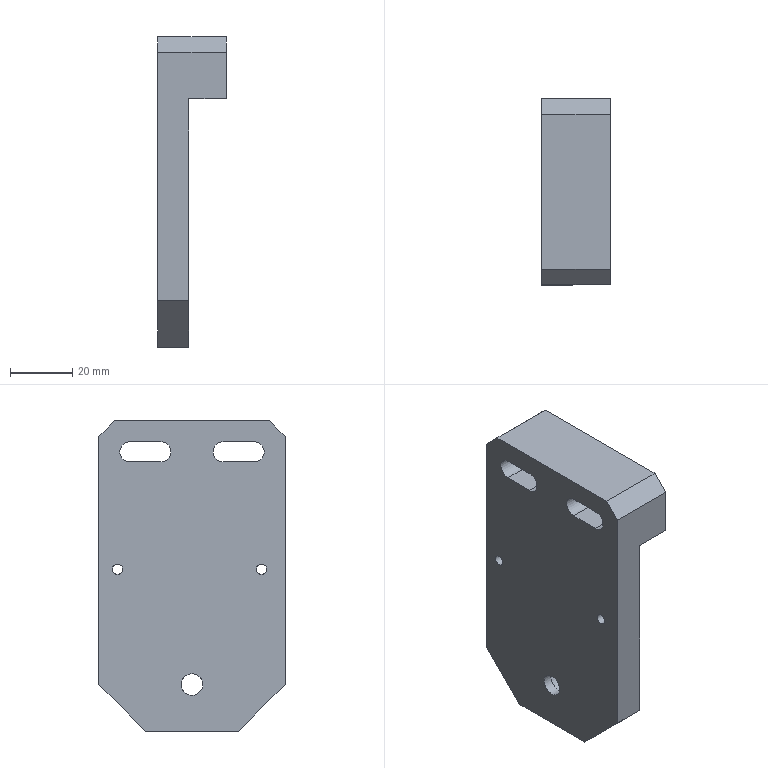Part | NX | features 5003_205_Bracket 2 | 1 solid | 25 faces | box 22 x 60 x 100 mm | volume 66444 mm3 | plane 17 | cylinder 8 | commonest cylinder face diameters 6.5 x4 3.3 x2 7 x1 10 x1
STEP:
#1=CARTESIAN_POINT('',(-243.475,-529.5,-147.));
#2=VERTEX_POINT('',#1);
#3=CARTESIAN_POINT('',(-243.475,-526.,-147.));
#4=DIRECTION('',(-1.,0.,0.));
#5=DIRECTION('',(0.,-1.,0.));
#6=AXIS2_PLACEMENT_3D('',#3,#4,#5);
#7=CIRCLE('',#6,3.5);
#8=EDGE_CURVE('',#2,#2,#7,.T.);
#9=ORIENTED_EDGE('',*,*,#8,.T.);
#10=EDGE_LOOP('',(#9));
#11=FACE_BOUND('',#10,.T.);
#12=CARTESIAN_POINT('',(-240.475,-526.,-143.5));
#13=VERTEX_POINT('',#12);
#14=CARTESIAN_POINT('',(-240.475,-526.,-147.));
#15=DIRECTION('',(1.,0.,0.));
#16=DIRECTION('',(0.,0.,1.));
#17=AXIS2_PLACEMENT_3D('',#14,#15,#16);
#18=CIRCLE('',#17,3.5);
#19=EDGE_CURVE('',#13,#13,#18,.T.);
#20=ORIENTED_EDGE('',*,*,#19,.T.);
#21=EDGE_LOOP('',(#20));
#22=FACE_BOUND('',#21,.T.);
#23=CARTESIAN_POINT('',(-243.475,-526.,-147.));
#24=DIRECTION('',(1.,0.,0.));
#25=DIRECTION('',(0.,1.,0.));
#26=AXIS2_PLACEMENT_3D('',#23,#24,#25);
#27=CYLINDRICAL_SURFACE('',#26,3.5);
#28=ADVANCED_FACE('',(#11,#22),#27,.F.);
#29=CARTESIAN_POINT('',(-243.475,-503.65,-109.85));
#30=VERTEX_POINT('',#29);
#31=CARTESIAN_POINT('',(-243.475,-502.,-109.85));
#32=DIRECTION('',(-1.,0.,0.));
#33=DIRECTION('',(0.,-1.,0.));
#34=AXIS2_PLACEMENT_3D('',#31,#32,#33);
#35=CIRCLE('',#34,1.65);
#36=EDGE_CURVE('',#30,#30,#35,.T.);
#37=ORIENTED_EDGE('',*,*,#36,.F.);
#38=EDGE_LOOP('',(#37));
#39=FACE_BOUND('',#38,.T.);
#40=CARTESIAN_POINT('',(-243.475,-550.05,-109.85));
#41=VERTEX_POINT('',#40);
#42=CARTESIAN_POINT('',(-243.475,-548.4,-109.85));
#43=DIRECTION('',(-1.,0.,0.));
#44=DIRECTION('',(0.,-1.,0.));
#45=AXIS2_PLACEMENT_3D('',#42,#43,#44);
#46=CIRCLE('',#45,1.65);
#47=EDGE_CURVE('',#41,#41,#46,.T.);
#48=ORIENTED_EDGE('',*,*,#47,.F.);
#49=EDGE_LOOP('',(#48));
#50=FACE_BOUND('',#49,.T.);
#51=CARTESIAN_POINT('',(-243.475,-551.,-62.));
#52=VERTEX_POINT('',#51);
#53=CARTESIAN_POINT('',(-243.475,-501.,-62.));
#54=VERTEX_POINT('',#53);
#55=CARTESIAN_POINT('',(-243.475,-496.,-62.));
#56=DIRECTION('',(0.,1.,0.));
#57=VECTOR('',#56,1000.);
#58=LINE('',#55,#57);
#59=EDGE_CURVE('',#52,#54,#58,.T.);
#60=ORIENTED_EDGE('',*,*,#59,.T.);
#61=CARTESIAN_POINT('',(-243.475,-496.,-67.));
#62=VERTEX_POINT('',#61);
#63=CARTESIAN_POINT('',(-243.475,-414.498,-148.502));
#64=DIRECTION('',(0.,-0.7071,0.7071));
#65=VECTOR('',#64,1000.);
#66=LINE('',#63,#65);
#67=EDGE_CURVE('',#54,#62,#66,.F.);
#68=ORIENTED_EDGE('',*,*,#67,.T.);
#69=CARTESIAN_POINT('',(-243.475,-496.,-147.));
#70=VERTEX_POINT('',#69);
#71=CARTESIAN_POINT('',(-243.475,-496.,-62.));
#72=DIRECTION('',(0.,0.,-1.));
#73=VECTOR('',#72,1000.);
#74=LINE('',#71,#73);
#75=EDGE_CURVE('',#62,#70,#74,.T.);
#76=ORIENTED_EDGE('',*,*,#75,.T.);
#77=CARTESIAN_POINT('',(-243.475,-511.,-162.));
#78=VERTEX_POINT('',#77);
#79=CARTESIAN_POINT('',(-243.475,-496.,-147.));
#80=DIRECTION('',(0.,-0.7071,-0.7071));
#81=VECTOR('',#80,1000.);
#82=LINE('',#79,#81);
#83=EDGE_CURVE('',#70,#78,#82,.T.);
#84=ORIENTED_EDGE('',*,*,#83,.T.);
#85=CARTESIAN_POINT('',(-243.475,-541.,-162.));
#86=VERTEX_POINT('',#85);
#87=CARTESIAN_POINT('',(-243.475,-511.,-162.));
#88=DIRECTION('',(0.,-1.,0.));
#89=VECTOR('',#88,1000.);
#90=LINE('',#87,#89);
#91=EDGE_CURVE('',#78,#86,#90,.T.);
#92=ORIENTED_EDGE('',*,*,#91,.T.);
#93=CARTESIAN_POINT('',(-243.475,-556.,-147.));
#94=VERTEX_POINT('',#93);
#95=CARTESIAN_POINT('',(-243.475,-541.,-162.));
#96=DIRECTION('',(0.,-0.7071,0.7071));
#97=VECTOR('',#96,1000.);
#98=LINE('',#95,#97);
#99=EDGE_CURVE('',#86,#94,#98,.T.);
#100=ORIENTED_EDGE('',*,*,#99,.T.);
#101=CARTESIAN_POINT('',(-243.475,-556.,-67.));
#102=VERTEX_POINT('',#101);
#103=CARTESIAN_POINT('',(-243.475,-556.,-62.));
#104=DIRECTION('',(0.,0.,1.));
#105=VECTOR('',#104,1000.);
#106=LINE('',#103,#105);
#107=EDGE_CURVE('',#94,#102,#106,.T.);
#108=ORIENTED_EDGE('',*,*,#107,.T.);
#109=CARTESIAN_POINT('',(-243.475,-615.498,-126.498));
#110=DIRECTION('',(0.,-0.7071,-0.7071));
#111=VECTOR('',#110,1000.);
#112=LINE('',#109,#111);
#113=EDGE_CURVE('',#102,#52,#112,.F.);
#114=ORIENTED_EDGE('',*,*,#113,.T.);
#115=EDGE_LOOP('',(#60,#68,#76,#84,#92,#100,#108,#114));
#116=FACE_BOUND('',#115,.T.);
#117=ORIENTED_EDGE('',*,*,#8,.F.);
#118=EDGE_LOOP('',(#117));
#119=FACE_BOUND('',#118,.T.);
#120=CARTESIAN_POINT('',(-243.475,-506.,-75.25));
#121=VERTEX_POINT('',#120);
#122=CARTESIAN_POINT('',(-243.475,-516.,-75.25));
#123=VERTEX_POINT('',#122);
#124=CARTESIAN_POINT('',(-243.475,-506.,-75.25));
#125=DIRECTION('',(0.,-1.,0.));
#126=VECTOR('',#125,1000.);
#127=LINE('',#124,#126);
#128=EDGE_CURVE('',#121,#123,#127,.T.);
#129=ORIENTED_EDGE('',*,*,#128,.F.);
#130=CARTESIAN_POINT('',(-243.475,-506.,-68.75));
#131=VERTEX_POINT('',#130);
#132=CARTESIAN_POINT('',(-243.475,-506.,-72.));
#133=DIRECTION('',(-1.,0.,0.));
#134=DIRECTION('',(0.,-1.,0.));
#135=AXIS2_PLACEMENT_3D('',#132,#133,#134);
#136=CIRCLE('',#135,3.25);
#137=EDGE_CURVE('',#131,#121,#136,.T.);
#138=ORIENTED_EDGE('',*,*,#137,.F.);
#139=CARTESIAN_POINT('',(-243.475,-516.,-68.75));
#140=VERTEX_POINT('',#139);
#141=CARTESIAN_POINT('',(-243.475,-506.,-68.75));
#142=DIRECTION('',(0.,1.,0.));
#143=VECTOR('',#142,1000.);
#144=LINE('',#141,#143);
#145=EDGE_CURVE('',#140,#131,#144,.T.);
#146=ORIENTED_EDGE('',*,*,#145,.F.);
#147=CARTESIAN_POINT('',(-243.475,-516.,-72.));
#148=DIRECTION('',(-1.,0.,0.));
#149=DIRECTION('',(0.,-1.,0.));
#150=AXIS2_PLACEMENT_3D('',#147,#148,#149);
#151=CIRCLE('',#150,3.25);
#152=EDGE_CURVE('',#123,#140,#151,.T.);
#153=ORIENTED_EDGE('',*,*,#152,.F.);
#154=EDGE_LOOP('',(#129,#138,#146,#153));
#155=FACE_BOUND('',#154,.T.);
#156=CARTESIAN_POINT('',(-243.475,-536.,-75.25));
#157=VERTEX_POINT('',#156);
#158=CARTESIAN_POINT('',(-243.475,-546.,-75.25));
#159=VERTEX_POINT('',#158);
#160=CARTESIAN_POINT('',(-243.475,-536.,-75.25));
#161=DIRECTION('',(0.,-1.,0.));
#162=VECTOR('',#161,1000.);
#163=LINE('',#160,#162);
#164=EDGE_CURVE('',#157,#159,#163,.T.);
#165=ORIENTED_EDGE('',*,*,#164,.F.);
#166=CARTESIAN_POINT('',(-243.475,-536.,-68.75));
#167=VERTEX_POINT('',#166);
#168=CARTESIAN_POINT('',(-243.475,-536.,-72.));
#169=DIRECTION('',(-1.,0.,0.));
#170=DIRECTION('',(0.,-1.,0.));
#171=AXIS2_PLACEMENT_3D('',#168,#169,#170);
#172=CIRCLE('',#171,3.25);
#173=EDGE_CURVE('',#167,#157,#172,.T.);
#174=ORIENTED_EDGE('',*,*,#173,.F.);
#175=CARTESIAN_POINT('',(-243.475,-546.,-68.75));
#176=VERTEX_POINT('',#175);
#177=CARTESIAN_POINT('',(-243.475,-536.,-68.75));
#178=DIRECTION('',(0.,1.,0.));
#179=VECTOR('',#178,1000.);
#180=LINE('',#177,#179);
#181=EDGE_CURVE('',#176,#167,#180,.T.);
#182=ORIENTED_EDGE('',*,*,#181,.F.);
#183=CARTESIAN_POINT('',(-243.475,-546.,-72.));
#184=DIRECTION('',(-1.,0.,0.));
#185=DIRECTION('',(0.,-1.,0.));
#186=AXIS2_PLACEMENT_3D('',#183,#184,#185);
#187=CIRCLE('',#186,3.25);
#188=EDGE_CURVE('',#159,#176,#187,.T.);
#189=ORIENTED_EDGE('',*,*,#188,.F.);
#190=EDGE_LOOP('',(#165,#174,#182,#189));
#191=FACE_BOUND('',#190,.T.);
#192=CARTESIAN_POINT('',(-243.475,-503.996,-238.));
#193=DIRECTION('',(-1.,0.,0.));
#194=DIRECTION('',(0.,-1.,0.));
#195=AXIS2_PLACEMENT_3D('',#192,#193,#194);
#196=PLANE('',#195);
#197=ADVANCED_FACE('',(#39,#50,#116,#119,#155,#191),#196,.T.);
#198=CARTESIAN_POINT('',(-221.475,-506.,-68.75));
#199=VERTEX_POINT('',#198);
#200=CARTESIAN_POINT('',(-221.475,-506.,-75.25));
#201=VERTEX_POINT('',#200);
#202=CARTESIAN_POINT('',(-221.475,-506.,-72.));
#203=DIRECTION('',(-1.,0.,0.));
#204=DIRECTION('',(0.,-1.,0.));
#205=AXIS2_PLACEMENT_3D('',#202,#203,#204);
#206=CIRCLE('',#205,3.25);
#207=EDGE_CURVE('',#199,#201,#206,.T.);
#208=ORIENTED_EDGE('',*,*,#207,.T.);
#209=CARTESIAN_POINT('',(-221.475,-516.,-75.25));
#210=VERTEX_POINT('',#209);
#211=CARTESIAN_POINT('',(-221.475,-506.,-75.25));
#212=DIRECTION('',(0.,-1.,0.));
#213=VECTOR('',#212,1000.);
#214=LINE('',#211,#213);
#215=EDGE_CURVE('',#201,#210,#214,.T.);
#216=ORIENTED_EDGE('',*,*,#215,.T.);
#217=CARTESIAN_POINT('',(-221.475,-516.,-68.75));
#218=VERTEX_POINT('',#217);
#219=CARTESIAN_POINT('',(-221.475,-516.,-72.));
#220=DIRECTION('',(-1.,0.,0.));
#221=DIRECTION('',(0.,-1.,0.));
#222=AXIS2_PLACEMENT_3D('',#219,#220,#221);
#223=CIRCLE('',#222,3.25);
#224=EDGE_CURVE('',#210,#218,#223,.T.);
#225=ORIENTED_EDGE('',*,*,#224,.T.);
#226=CARTESIAN_POINT('',(-221.475,-506.,-68.75));
#227=DIRECTION('',(0.,1.,0.));
#228=VECTOR('',#227,1000.);
#229=LINE('',#226,#228);
#230=EDGE_CURVE('',#218,#199,#229,.T.);
#231=ORIENTED_EDGE('',*,*,#230,.T.);
#232=EDGE_LOOP('',(#208,#216,#225,#231));
#233=FACE_BOUND('',#232,.T.);
#234=CARTESIAN_POINT('',(-221.475,-496.,-67.));
#235=VERTEX_POINT('',#234);
#236=CARTESIAN_POINT('',(-221.475,-496.,-82.));
#237=VERTEX_POINT('',#236);
#238=CARTESIAN_POINT('',(-221.475,-496.,-62.));
#239=DIRECTION('',(0.,0.,-1.));
#240=VECTOR('',#239,1000.);
#241=LINE('',#238,#240);
#242=EDGE_CURVE('',#235,#237,#241,.T.);
#243=ORIENTED_EDGE('',*,*,#242,.F.);
#244=CARTESIAN_POINT('',(-221.475,-501.,-62.));
#245=VERTEX_POINT('',#244);
#246=CARTESIAN_POINT('',(-221.475,-496.,-67.));
#247=DIRECTION('',(0.,0.7071,-0.7071));
#248=VECTOR('',#247,1000.);
#249=LINE('',#246,#248);
#250=EDGE_CURVE('',#235,#245,#249,.F.);
#251=ORIENTED_EDGE('',*,*,#250,.T.);
#252=CARTESIAN_POINT('',(-221.475,-551.,-62.));
#253=VERTEX_POINT('',#252);
#254=CARTESIAN_POINT('',(-221.475,-496.,-62.));
#255=DIRECTION('',(0.,1.,0.));
#256=VECTOR('',#255,1000.);
#257=LINE('',#254,#256);
#258=EDGE_CURVE('',#253,#245,#257,.T.);
#259=ORIENTED_EDGE('',*,*,#258,.F.);
#260=CARTESIAN_POINT('',(-221.475,-556.,-67.));
#261=VERTEX_POINT('',#260);
#262=CARTESIAN_POINT('',(-221.475,-551.,-62.));
#263=DIRECTION('',(0.,0.7071,0.7071));
#264=VECTOR('',#263,1000.);
#265=LINE('',#262,#264);
#266=EDGE_CURVE('',#253,#261,#265,.F.);
#267=ORIENTED_EDGE('',*,*,#266,.T.);
#268=CARTESIAN_POINT('',(-221.475,-556.,-82.));
#269=VERTEX_POINT('',#268);
#270=CARTESIAN_POINT('',(-221.475,-556.,-62.));
#271=DIRECTION('',(0.,0.,1.));
#272=VECTOR('',#271,1000.);
#273=LINE('',#270,#272);
#274=EDGE_CURVE('',#269,#261,#273,.T.);
#275=ORIENTED_EDGE('',*,*,#274,.F.);
#276=CARTESIAN_POINT('',(-221.475,-495.999,-82.));
#277=DIRECTION('',(0.,-1.,0.));
#278=VECTOR('',#277,1000.);
#279=LINE('',#276,#278);
#280=EDGE_CURVE('',#237,#269,#279,.T.);
#281=ORIENTED_EDGE('',*,*,#280,.F.);
#282=EDGE_LOOP('',(#243,#251,#259,#267,#275,#281));
#283=FACE_BOUND('',#282,.T.);
#284=CARTESIAN_POINT('',(-221.475,-536.,-68.75));
#285=VERTEX_POINT('',#284);
#286=CARTESIAN_POINT('',(-221.475,-536.,-75.25));
#287=VERTEX_POINT('',#286);
#288=CARTESIAN_POINT('',(-221.475,-536.,-72.));
#289=DIRECTION('',(-1.,0.,0.));
#290=DIRECTION('',(0.,-1.,0.));
#291=AXIS2_PLACEMENT_3D('',#288,#289,#290);
#292=CIRCLE('',#291,3.25);
#293=EDGE_CURVE('',#285,#287,#292,.T.);
#294=ORIENTED_EDGE('',*,*,#293,.T.);
#295=CARTESIAN_POINT('',(-221.475,-546.,-75.25));
#296=VERTEX_POINT('',#295);
#297=CARTESIAN_POINT('',(-221.475,-536.,-75.25));
#298=DIRECTION('',(0.,-1.,0.));
#299=VECTOR('',#298,1000.);
#300=LINE('',#297,#299);
#301=EDGE_CURVE('',#287,#296,#300,.T.);
#302=ORIENTED_EDGE('',*,*,#301,.T.);
#303=CARTESIAN_POINT('',(-221.475,-546.,-68.75));
#304=VERTEX_POINT('',#303);
#305=CARTESIAN_POINT('',(-221.475,-546.,-72.));
#306=DIRECTION('',(-1.,0.,0.));
#307=DIRECTION('',(0.,-1.,0.));
#308=AXIS2_PLACEMENT_3D('',#305,#306,#307);
#309=CIRCLE('',#308,3.25);
#310=EDGE_CURVE('',#296,#304,#309,.T.);
#311=ORIENTED_EDGE('',*,*,#310,.T.);
#312=CARTESIAN_POINT('',(-221.475,-536.,-68.75));
#313=DIRECTION('',(0.,1.,0.));
#314=VECTOR('',#313,1000.);
#315=LINE('',#312,#314);
#316=EDGE_CURVE('',#304,#285,#315,.T.);
#317=ORIENTED_EDGE('',*,*,#316,.T.);
#318=EDGE_LOOP('',(#294,#302,#311,#317));
#319=FACE_BOUND('',#318,.T.);
#320=CARTESIAN_POINT('',(-221.475,-503.996,-238.));
#321=DIRECTION('',(-1.,0.,0.));
#322=DIRECTION('',(0.,-1.,0.));
#323=AXIS2_PLACEMENT_3D('',#320,#321,#322);
#324=PLANE('',#323);
#325=ADVANCED_FACE('',(#233,#283,#319),#324,.F.);
#326=ORIENTED_EDGE('',*,*,#75,.F.);
#327=CARTESIAN_POINT('',(-243.475,-496.,-67.));
#328=DIRECTION('',(1.,0.,0.));
#329=VECTOR('',#328,1000.);
#330=LINE('',#327,#329);
#331=EDGE_CURVE('',#62,#235,#330,.T.);
#332=ORIENTED_EDGE('',*,*,#331,.T.);
#333=ORIENTED_EDGE('',*,*,#242,.T.);
#334=CARTESIAN_POINT('',(-233.475,-496.,-82.));
#335=VERTEX_POINT('',#334);
#336=CARTESIAN_POINT('',(-233.475,-496.,-82.));
#337=DIRECTION('',(1.,0.,0.));
#338=VECTOR('',#337,1000.);
#339=LINE('',#336,#338);
#340=EDGE_CURVE('',#335,#237,#339,.T.);
#341=ORIENTED_EDGE('',*,*,#340,.F.);
#342=CARTESIAN_POINT('',(-233.475,-496.,-147.));
#343=VERTEX_POINT('',#342);
#344=CARTESIAN_POINT('',(-233.475,-496.,-82.));
#345=DIRECTION('',(0.,0.,1.));
#346=VECTOR('',#345,1000.);
#347=LINE('',#344,#346);
#348=EDGE_CURVE('',#343,#335,#347,.T.);
#349=ORIENTED_EDGE('',*,*,#348,.F.);
#350=CARTESIAN_POINT('',(-243.475,-496.,-147.));
#351=DIRECTION('',(1.,0.,0.));
#352=VECTOR('',#351,1000.);
#353=LINE('',#350,#352);
#354=EDGE_CURVE('',#70,#343,#353,.T.);
#355=ORIENTED_EDGE('',*,*,#354,.F.);
#356=EDGE_LOOP('',(#326,#332,#333,#341,#349,#355));
#357=FACE_BOUND('',#356,.T.);
#358=CARTESIAN_POINT('',(-243.475,-496.,-62.));
#359=DIRECTION('',(0.,-1.,0.));
#360=DIRECTION('',(0.,0.,1.));
#361=AXIS2_PLACEMENT_3D('',#358,#359,#360);
#362=PLANE('',#361);
#363=ADVANCED_FACE('',(#357),#362,.F.);
#364=ORIENTED_EDGE('',*,*,#354,.T.);
#365=CARTESIAN_POINT('',(-233.475,-511.,-162.));
#366=VERTEX_POINT('',#365);
#367=CARTESIAN_POINT('',(-233.475,-463.499,-114.499));
#368=DIRECTION('',(0.,0.7071,0.7071));
#369=VECTOR('',#368,1000.);
#370=LINE('',#367,#369);
#371=EDGE_CURVE('',#366,#343,#370,.T.);
#372=ORIENTED_EDGE('',*,*,#371,.F.);
#373=CARTESIAN_POINT('',(-243.475,-511.,-162.));
#374=DIRECTION('',(1.,0.,0.));
#375=VECTOR('',#374,1000.);
#376=LINE('',#373,#375);
#377=EDGE_CURVE('',#78,#366,#376,.T.);
#378=ORIENTED_EDGE('',*,*,#377,.F.);
#379=ORIENTED_EDGE('',*,*,#83,.F.);
#380=EDGE_LOOP('',(#364,#372,#378,#379));
#381=FACE_BOUND('',#380,.T.);
#382=CARTESIAN_POINT('',(-243.475,-496.,-147.));
#383=DIRECTION('',(0.,-0.7071,0.7071));
#384=DIRECTION('',(0.,0.7071,0.7071));
#385=AXIS2_PLACEMENT_3D('',#382,#383,#384);
#386=PLANE('',#385);
#387=ADVANCED_FACE('',(#381),#386,.F.);
#388=ORIENTED_EDGE('',*,*,#377,.T.);
#389=CARTESIAN_POINT('',(-233.475,-541.,-162.));
#390=VERTEX_POINT('',#389);
#391=CARTESIAN_POINT('',(-233.475,-495.999,-162.));
#392=DIRECTION('',(0.,-1.,0.));
#393=VECTOR('',#392,1000.);
#394=LINE('',#391,#393);
#395=EDGE_CURVE('',#366,#390,#394,.T.);
#396=ORIENTED_EDGE('',*,*,#395,.T.);
#397=CARTESIAN_POINT('',(-243.475,-541.,-162.));
#398=DIRECTION('',(1.,0.,0.));
#399=VECTOR('',#398,1000.);
#400=LINE('',#397,#399);
#401=EDGE_CURVE('',#86,#390,#400,.T.);
#402=ORIENTED_EDGE('',*,*,#401,.F.);
#403=ORIENTED_EDGE('',*,*,#91,.F.);
#404=EDGE_LOOP('',(#388,#396,#402,#403));
#405=FACE_BOUND('',#404,.T.);
#406=CARTESIAN_POINT('',(-243.475,-511.,-162.));
#407=DIRECTION('',(0.,0.,1.));
#408=DIRECTION('',(-1.,0.,0.));
#409=AXIS2_PLACEMENT_3D('',#406,#407,#408);
#410=PLANE('',#409);
#411=ADVANCED_FACE('',(#405),#410,.F.);
#412=ORIENTED_EDGE('',*,*,#401,.T.);
#413=CARTESIAN_POINT('',(-233.475,-556.,-147.));
#414=VERTEX_POINT('',#413);
#415=CARTESIAN_POINT('',(-233.475,-558.499,-144.5));
#416=DIRECTION('',(0.,0.7071,-0.7071));
#417=VECTOR('',#416,1000.);
#418=LINE('',#415,#417);
#419=EDGE_CURVE('',#414,#390,#418,.T.);
#420=ORIENTED_EDGE('',*,*,#419,.F.);
#421=CARTESIAN_POINT('',(-243.475,-556.,-147.));
#422=DIRECTION('',(1.,0.,0.));
#423=VECTOR('',#422,1000.);
#424=LINE('',#421,#423);
#425=EDGE_CURVE('',#94,#414,#424,.T.);
#426=ORIENTED_EDGE('',*,*,#425,.F.);
#427=ORIENTED_EDGE('',*,*,#99,.F.);
#428=EDGE_LOOP('',(#412,#420,#426,#427));
#429=FACE_BOUND('',#428,.T.);
#430=CARTESIAN_POINT('',(-243.475,-541.,-162.));
#431=DIRECTION('',(0.,0.7071,0.7071));
#432=DIRECTION('',(0.,0.7071,-0.7071));
#433=AXIS2_PLACEMENT_3D('',#430,#431,#432);
#434=PLANE('',#433);
#435=ADVANCED_FACE('',(#429),#434,.F.);
#436=ORIENTED_EDGE('',*,*,#274,.T.);
#437=CARTESIAN_POINT('',(-243.475,-556.,-67.));
#438=DIRECTION('',(-1.,0.,0.));
#439=VECTOR('',#438,1000.);
#440=LINE('',#437,#439);
#441=EDGE_CURVE('',#261,#102,#440,.T.);
#442=ORIENTED_EDGE('',*,*,#441,.T.);
#443=ORIENTED_EDGE('',*,*,#107,.F.);
#444=ORIENTED_EDGE('',*,*,#425,.T.);
#445=CARTESIAN_POINT('',(-233.475,-556.,-82.));
#446=VERTEX_POINT('',#445);
#447=CARTESIAN_POINT('',(-233.475,-556.,-82.));
#448=DIRECTION('',(0.,0.,-1.));
#449=VECTOR('',#448,1000.);
#450=LINE('',#447,#449);
#451=EDGE_CURVE('',#446,#414,#450,.T.);
#452=ORIENTED_EDGE('',*,*,#451,.F.);
#453=CARTESIAN_POINT('',(-233.475,-556.,-82.));
#454=DIRECTION('',(-1.,0.,0.));
#455=VECTOR('',#454,1000.);
#456=LINE('',#453,#455);
#457=EDGE_CURVE('',#269,#446,#456,.T.);
#458=ORIENTED_EDGE('',*,*,#457,.F.);
#459=EDGE_LOOP('',(#436,#442,#443,#444,#452,#458));
#460=FACE_BOUND('',#459,.T.);
#461=CARTESIAN_POINT('',(-243.475,-556.,-62.));
#462=DIRECTION('',(0.,1.,0.));
#463=DIRECTION('',(0.,0.,-1.));
#464=AXIS2_PLACEMENT_3D('',#461,#462,#463);
#465=PLANE('',#464);
#466=ADVANCED_FACE('',(#460),#465,.F.);
#467=ORIENTED_EDGE('',*,*,#258,.T.);
#468=CARTESIAN_POINT('',(-243.475,-501.,-62.));
#469=DIRECTION('',(-1.,0.,0.));
#470=VECTOR('',#469,1000.);
#471=LINE('',#468,#470);
#472=EDGE_CURVE('',#245,#54,#471,.T.);
#473=ORIENTED_EDGE('',*,*,#472,.T.);
#474=ORIENTED_EDGE('',*,*,#59,.F.);
#475=CARTESIAN_POINT('',(-243.475,-551.,-62.));
#476=DIRECTION('',(1.,0.,0.));
#477=VECTOR('',#476,1000.);
#478=LINE('',#475,#477);
#479=EDGE_CURVE('',#52,#253,#478,.T.);
#480=ORIENTED_EDGE('',*,*,#479,.T.);
#481=EDGE_LOOP('',(#467,#473,#474,#480));
#482=FACE_BOUND('',#481,.T.);
#483=CARTESIAN_POINT('',(-243.475,-496.,-62.));
#484=DIRECTION('',(0.,0.,-1.));
#485=DIRECTION('',(1.,0.,0.));
#486=AXIS2_PLACEMENT_3D('',#483,#484,#485);
#487=PLANE('',#486);
#488=ADVANCED_FACE('',(#482),#487,.F.);
#489=ORIENTED_EDGE('',*,*,#207,.F.);
#490=CARTESIAN_POINT('',(-243.475,-506.,-68.75));
#491=DIRECTION('',(1.,0.,0.));
#492=VECTOR('',#491,1000.);
#493=LINE('',#490,#492);
#494=EDGE_CURVE('',#131,#199,#493,.T.);
#495=ORIENTED_EDGE('',*,*,#494,.F.);
#496=ORIENTED_EDGE('',*,*,#137,.T.);
#497=CARTESIAN_POINT('',(-243.475,-506.,-75.25));
#498=DIRECTION('',(1.,0.,0.));
#499=VECTOR('',#498,1000.);
#500=LINE('',#497,#499);
#501=EDGE_CURVE('',#121,#201,#500,.T.);
#502=ORIENTED_EDGE('',*,*,#501,.T.);
#503=EDGE_LOOP('',(#489,#495,#496,#502));
#504=FACE_BOUND('',#503,.T.);
#505=CARTESIAN_POINT('',(-243.475,-506.,-72.));
#506=DIRECTION('',(1.,0.,0.));
#507=DIRECTION('',(0.,1.,0.));
#508=AXIS2_PLACEMENT_3D('',#505,#506,#507);
#509=CYLINDRICAL_SURFACE('',#508,3.25);
#510=ADVANCED_FACE('',(#504),#509,.F.);
#511=ORIENTED_EDGE('',*,*,#215,.F.);
#512=ORIENTED_EDGE('',*,*,#501,.F.);
#513=ORIENTED_EDGE('',*,*,#128,.T.);
#514=CARTESIAN_POINT('',(-243.475,-516.,-75.25));
#515=DIRECTION('',(1.,0.,0.));
#516=VECTOR('',#515,1000.);
#517=LINE('',#514,#516);
#518=EDGE_CURVE('',#123,#210,#517,.T.);
#519=ORIENTED_EDGE('',*,*,#518,.T.);
#520=EDGE_LOOP('',(#511,#512,#513,#519));
#521=FACE_BOUND('',#520,.T.);
#522=CARTESIAN_POINT('',(-243.475,-506.,-75.25));
#523=DIRECTION('',(0.,0.,1.));
#524=DIRECTION('',(-1.,0.,0.));
#525=AXIS2_PLACEMENT_3D('',#522,#523,#524);
#526=PLANE('',#525);
#527=ADVANCED_FACE('',(#521),#526,.T.);
#528=ORIENTED_EDGE('',*,*,#224,.F.);
#529=ORIENTED_EDGE('',*,*,#518,.F.);
#530=ORIENTED_EDGE('',*,*,#152,.T.);
#531=CARTESIAN_POINT('',(-243.475,-516.,-68.75));
#532=DIRECTION('',(1.,0.,0.));
#533=VECTOR('',#532,1000.);
#534=LINE('',#531,#533);
#535=EDGE_CURVE('',#140,#218,#534,.T.);
#536=ORIENTED_EDGE('',*,*,#535,.T.);
#537=EDGE_LOOP('',(#528,#529,#530,#536));
#538=FACE_BOUND('',#537,.T.);
#539=CARTESIAN_POINT('',(-243.475,-516.,-72.));
#540=DIRECTION('',(1.,0.,0.));
#541=DIRECTION('',(0.,1.,0.));
#542=AXIS2_PLACEMENT_3D('',#539,#540,#541);
#543=CYLINDRICAL_SURFACE('',#542,3.25);
#544=ADVANCED_FACE('',(#538),#543,.F.);
#545=ORIENTED_EDGE('',*,*,#230,.F.);
#546=ORIENTED_EDGE('',*,*,#535,.F.);
#547=ORIENTED_EDGE('',*,*,#145,.T.);
#548=ORIENTED_EDGE('',*,*,#494,.T.);
#549=EDGE_LOOP('',(#545,#546,#547,#548));
#550=FACE_BOUND('',#549,.T.);
#551=CARTESIAN_POINT('',(-243.475,-506.,-68.75));
#552=DIRECTION('',(0.,0.,-1.));
#553=DIRECTION('',(1.,0.,0.));
#554=AXIS2_PLACEMENT_3D('',#551,#552,#553);
#555=PLANE('',#554);
#556=ADVANCED_FACE('',(#550),#555,.T.);
#557=ORIENTED_EDGE('',*,*,#293,.F.);
#558=CARTESIAN_POINT('',(-243.475,-536.,-68.75));
#559=DIRECTION('',(1.,0.,0.));
#560=VECTOR('',#559,1000.);
#561=LINE('',#558,#560);
#562=EDGE_CURVE('',#167,#285,#561,.T.);
#563=ORIENTED_EDGE('',*,*,#562,.F.);
#564=ORIENTED_EDGE('',*,*,#173,.T.);
#565=CARTESIAN_POINT('',(-243.475,-536.,-75.25));
#566=DIRECTION('',(1.,0.,0.));
#567=VECTOR('',#566,1000.);
#568=LINE('',#565,#567);
#569=EDGE_CURVE('',#157,#287,#568,.T.);
#570=ORIENTED_EDGE('',*,*,#569,.T.);
#571=EDGE_LOOP('',(#557,#563,#564,#570));
#572=FACE_BOUND('',#571,.T.);
#573=CARTESIAN_POINT('',(-243.475,-536.,-72.));
#574=DIRECTION('',(1.,0.,0.));
#575=DIRECTION('',(0.,1.,0.));
#576=AXIS2_PLACEMENT_3D('',#573,#574,#575);
#577=CYLINDRICAL_SURFACE('',#576,3.25);
#578=ADVANCED_FACE('',(#572),#577,.F.);
#579=ORIENTED_EDGE('',*,*,#301,.F.);
#580=ORIENTED_EDGE('',*,*,#569,.F.);
#581=ORIENTED_EDGE('',*,*,#164,.T.);
#582=CARTESIAN_POINT('',(-243.475,-546.,-75.25));
#583=DIRECTION('',(1.,0.,0.));
#584=VECTOR('',#583,1000.);
#585=LINE('',#582,#584);
#586=EDGE_CURVE('',#159,#296,#585,.T.);
#587=ORIENTED_EDGE('',*,*,#586,.T.);
#588=EDGE_LOOP('',(#579,#580,#581,#587));
#589=FACE_BOUND('',#588,.T.);
#590=CARTESIAN_POINT('',(-243.475,-536.,-75.25));
#591=DIRECTION('',(0.,0.,1.));
#592=DIRECTION('',(-1.,0.,0.));
#593=AXIS2_PLACEMENT_3D('',#590,#591,#592);
#594=PLANE('',#593);
#595=ADVANCED_FACE('',(#589),#594,.T.);
#596=ORIENTED_EDGE('',*,*,#310,.F.);
#597=ORIENTED_EDGE('',*,*,#586,.F.);
#598=ORIENTED_EDGE('',*,*,#188,.T.);
#599=CARTESIAN_POINT('',(-243.475,-546.,-68.75));
#600=DIRECTION('',(1.,0.,0.));
#601=VECTOR('',#600,1000.);
#602=LINE('',#599,#601);
#603=EDGE_CURVE('',#176,#304,#602,.T.);
#604=ORIENTED_EDGE('',*,*,#603,.T.);
#605=EDGE_LOOP('',(#596,#597,#598,#604));
#606=FACE_BOUND('',#605,.T.);
#607=CARTESIAN_POINT('',(-243.475,-546.,-72.));
#608=DIRECTION('',(1.,0.,0.));
#609=DIRECTION('',(0.,1.,0.));
#610=AXIS2_PLACEMENT_3D('',#607,#608,#609);
#611=CYLINDRICAL_SURFACE('',#610,3.25);
#612=ADVANCED_FACE('',(#606),#611,.F.);
#613=ORIENTED_EDGE('',*,*,#316,.F.);
#614=ORIENTED_EDGE('',*,*,#603,.F.);
#615=ORIENTED_EDGE('',*,*,#181,.T.);
#616=ORIENTED_EDGE('',*,*,#562,.T.);
#617=EDGE_LOOP('',(#613,#614,#615,#616));
#618=FACE_BOUND('',#617,.T.);
#619=CARTESIAN_POINT('',(-243.475,-536.,-68.75));
#620=DIRECTION('',(0.,0.,-1.));
#621=DIRECTION('',(1.,0.,0.));
#622=AXIS2_PLACEMENT_3D('',#619,#620,#621);
#623=PLANE('',#622);
#624=ADVANCED_FACE('',(#618),#623,.T.);
#625=CARTESIAN_POINT('',(-233.475,-502.,-111.5));
#626=VERTEX_POINT('',#625);
#627=CARTESIAN_POINT('',(-233.475,-502.,-109.85));
#628=DIRECTION('',(-1.,0.,0.));
#629=DIRECTION('',(0.,0.,-1.));
#630=AXIS2_PLACEMENT_3D('',#627,#628,#629);
#631=CIRCLE('',#630,1.65);
#632=EDGE_CURVE('',#626,#626,#631,.T.);
#633=ORIENTED_EDGE('',*,*,#632,.T.);
#634=EDGE_LOOP('',(#633));
#635=FACE_BOUND('',#634,.T.);
#636=CARTESIAN_POINT('',(-233.475,-548.4,-111.5));
#637=VERTEX_POINT('',#636);
#638=CARTESIAN_POINT('',(-233.475,-548.4,-109.85));
#639=DIRECTION('',(-1.,0.,0.));
#640=DIRECTION('',(0.,0.,-1.));
#641=AXIS2_PLACEMENT_3D('',#638,#639,#640);
#642=CIRCLE('',#641,1.65);
#643=EDGE_CURVE('',#637,#637,#642,.T.);
#644=ORIENTED_EDGE('',*,*,#643,.T.);
#645=EDGE_LOOP('',(#644));
#646=FACE_BOUND('',#645,.T.);
#647=CARTESIAN_POINT('',(-233.475,-526.,-142.));
#648=VERTEX_POINT('',#647);
#649=CARTESIAN_POINT('',(-233.475,-526.,-147.));
#650=DIRECTION('',(1.,0.,0.));
#651=DIRECTION('',(0.,0.,1.));
#652=AXIS2_PLACEMENT_3D('',#649,#650,#651);
#653=CIRCLE('',#652,5.);
#654=EDGE_CURVE('',#648,#648,#653,.T.);
#655=ORIENTED_EDGE('',*,*,#654,.F.);
#656=EDGE_LOOP('',(#655));
#657=FACE_BOUND('',#656,.T.);
#658=ORIENTED_EDGE('',*,*,#348,.T.);
#659=CARTESIAN_POINT('',(-233.475,-495.999,-82.));
#660=DIRECTION('',(0.,-1.,0.));
#661=VECTOR('',#660,1000.);
#662=LINE('',#659,#661);
#663=EDGE_CURVE('',#335,#446,#662,.T.);
#664=ORIENTED_EDGE('',*,*,#663,.T.);
#665=ORIENTED_EDGE('',*,*,#451,.T.);
#666=ORIENTED_EDGE('',*,*,#419,.T.);
#667=ORIENTED_EDGE('',*,*,#395,.F.);
#668=ORIENTED_EDGE('',*,*,#371,.T.);
#669=EDGE_LOOP('',(#658,#664,#665,#666,#667,#668));
#670=FACE_BOUND('',#669,.T.);
#671=CARTESIAN_POINT('',(-233.475,-495.999,-82.));
#672=DIRECTION('',(-1.,0.,0.));
#673=DIRECTION('',(0.,0.,-1.));
#674=AXIS2_PLACEMENT_3D('',#671,#672,#673);
#675=PLANE('',#674);
#676=ADVANCED_FACE('',(#635,#646,#657,#670),#675,.F.);
#677=ORIENTED_EDGE('',*,*,#340,.T.);
#678=ORIENTED_EDGE('',*,*,#280,.T.);
#679=ORIENTED_EDGE('',*,*,#457,.T.);
#680=ORIENTED_EDGE('',*,*,#663,.F.);
#681=EDGE_LOOP('',(#677,#678,#679,#680));
#682=FACE_BOUND('',#681,.T.);
#683=CARTESIAN_POINT('',(-233.475,-495.999,-82.));
#684=DIRECTION('',(0.,0.,1.));
#685=DIRECTION('',(0.,1.,0.));
#686=AXIS2_PLACEMENT_3D('',#683,#684,#685);
#687=PLANE('',#686);
#688=ADVANCED_FACE('',(#682),#687,.F.);
#689=CARTESIAN_POINT('',(-240.475,-526.,-142.));
#690=VERTEX_POINT('',#689);
#691=CARTESIAN_POINT('',(-240.475,-526.,-147.));
#692=DIRECTION('',(1.,0.,0.));
#693=DIRECTION('',(0.,0.,1.));
#694=AXIS2_PLACEMENT_3D('',#691,#692,#693);
#695=CIRCLE('',#694,5.);
#696=EDGE_CURVE('',#690,#690,#695,.T.);
#697=ORIENTED_EDGE('',*,*,#696,.F.);
#698=EDGE_LOOP('',(#697));
#699=FACE_BOUND('',#698,.T.);
#700=ORIENTED_EDGE('',*,*,#654,.T.);
#701=EDGE_LOOP('',(#700));
#702=FACE_BOUND('',#701,.T.);
#703=CARTESIAN_POINT('',(-240.475,-526.,-147.));
#704=DIRECTION('',(1.,0.,0.));
#705=DIRECTION('',(0.,0.,1.));
#706=AXIS2_PLACEMENT_3D('',#703,#704,#705);
#707=CYLINDRICAL_SURFACE('',#706,5.);
#708=ADVANCED_FACE('',(#699,#702),#707,.F.);
#709=ORIENTED_EDGE('',*,*,#19,.F.);
#710=EDGE_LOOP('',(#709));
#711=FACE_BOUND('',#710,.T.);
#712=ORIENTED_EDGE('',*,*,#696,.T.);
#713=EDGE_LOOP('',(#712));
#714=FACE_BOUND('',#713,.T.);
#715=CARTESIAN_POINT('',(-240.475,-526.,-147.));
#716=DIRECTION('',(1.,0.,0.));
#717=DIRECTION('',(0.,0.,1.));
#718=AXIS2_PLACEMENT_3D('',#715,#716,#717);
#719=PLANE('',#718);
#720=ADVANCED_FACE('',(#711,#714),#719,.T.);
#721=ORIENTED_EDGE('',*,*,#47,.T.);
#722=EDGE_LOOP('',(#721));
#723=FACE_BOUND('',#722,.T.);
#724=ORIENTED_EDGE('',*,*,#643,.F.);
#725=EDGE_LOOP('',(#724));
#726=FACE_BOUND('',#725,.T.);
#727=CARTESIAN_POINT('',(-243.475,-548.4,-109.85));
#728=DIRECTION('',(-1.,0.,0.));
#729=DIRECTION('',(0.,-1.,0.));
#730=AXIS2_PLACEMENT_3D('',#727,#728,#729);
#731=CYLINDRICAL_SURFACE('',#730,1.65);
#732=ADVANCED_FACE('',(#723,#726),#731,.F.);
#733=ORIENTED_EDGE('',*,*,#36,.T.);
#734=EDGE_LOOP('',(#733));
#735=FACE_BOUND('',#734,.T.);
#736=ORIENTED_EDGE('',*,*,#632,.F.);
#737=EDGE_LOOP('',(#736));
#738=FACE_BOUND('',#737,.T.);
#739=CARTESIAN_POINT('',(-243.475,-502.,-109.85));
#740=DIRECTION('',(-1.,0.,0.));
#741=DIRECTION('',(0.,-1.,0.));
#742=AXIS2_PLACEMENT_3D('',#739,#740,#741);
#743=CYLINDRICAL_SURFACE('',#742,1.65);
#744=ADVANCED_FACE('',(#735,#738),#743,.F.);
#745=ORIENTED_EDGE('',*,*,#67,.F.);
#746=ORIENTED_EDGE('',*,*,#472,.F.);
#747=ORIENTED_EDGE('',*,*,#250,.F.);
#748=ORIENTED_EDGE('',*,*,#331,.F.);
#749=EDGE_LOOP('',(#745,#746,#747,#748));
#750=FACE_BOUND('',#749,.T.);
#751=CARTESIAN_POINT('',(-243.475,-496.,-67.));
#752=DIRECTION('',(0.,-0.7071,-0.7071));
#753=DIRECTION('',(1.,0.,0.));
#754=AXIS2_PLACEMENT_3D('',#751,#752,#753);
#755=PLANE('',#754);
#756=ADVANCED_FACE('',(#750),#755,.F.);
#757=ORIENTED_EDGE('',*,*,#113,.F.);
#758=ORIENTED_EDGE('',*,*,#441,.F.);
#759=ORIENTED_EDGE('',*,*,#266,.F.);
#760=ORIENTED_EDGE('',*,*,#479,.F.);
#761=EDGE_LOOP('',(#757,#758,#759,#760));
#762=FACE_BOUND('',#761,.T.);
#763=CARTESIAN_POINT('',(-243.475,-551.,-62.));
#764=DIRECTION('',(0.,0.7071,-0.7071));
#765=DIRECTION('',(1.,0.,0.));
#766=AXIS2_PLACEMENT_3D('',#763,#764,#765);
#767=PLANE('',#766);
#768=ADVANCED_FACE('',(#762),#767,.F.);
#769=CLOSED_SHELL('',(#28,#197,#325,#363,#387,#411,#435,#466,#488,#510,#527,#544,#556,#578,#595,#612,#624,#676,#688,#708,#720,#732,#744,#756,#768));
#770=MANIFOLD_SOLID_BREP('',#769);
#771=(LENGTH_UNIT()NAMED_UNIT(*)SI_UNIT(.MILLI.,.METRE.));
#772=UNCERTAINTY_MEASURE_WITH_UNIT(LENGTH_MEASURE(0.00001),#771,'','');
#773=(NAMED_UNIT(*)PLANE_ANGLE_UNIT()SI_UNIT($,.RADIAN.));
#774=(NAMED_UNIT(*)SI_UNIT($,.STERADIAN.)SOLID_ANGLE_UNIT());
#775=(GEOMETRIC_REPRESENTATION_CONTEXT(3)GLOBAL_UNCERTAINTY_ASSIGNED_CONTEXT((#772))GLOBAL_UNIT_ASSIGNED_CONTEXT((#771,#773,#774))REPRESENTATION_CONTEXT('',''));
#776=ADVANCED_BREP_SHAPE_REPRESENTATION('',(#770),#775);